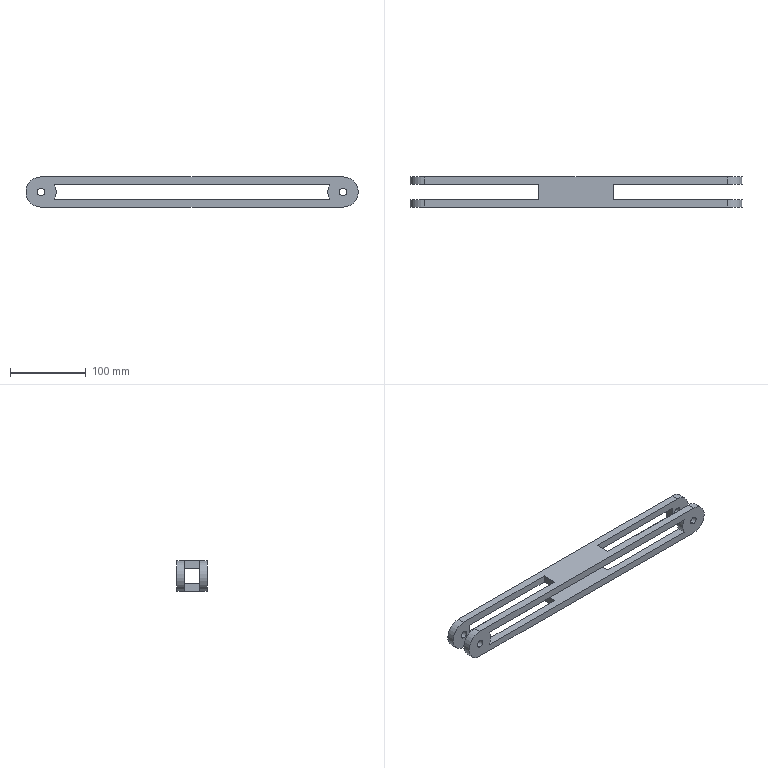Part | SolidWorks | features ICE 4, MirrorPattern 2, Extrusion 1 | 1 solid | 30 faces | box 440 x 40 x 40 mm | volume 233504 mm3 | plane 16 | cylinder 14 | commonest cylinder face diameters 10 x8 40 x6
STEP:
#1=CARTESIAN_POINT('',(-200.,-20.,-5.));
#2=VERTEX_POINT('',#1);
#3=CARTESIAN_POINT('',(-200.,-20.,5.));
#4=VERTEX_POINT('',#3);
#5=CARTESIAN_POINT('',(-200.,-20.,0.));
#6=DIRECTION('',(0.,1.,0.));
#7=DIRECTION('',(0.,0.,-1.));
#8=AXIS2_PLACEMENT_3D('',#5,#6,#7);
#9=CIRCLE('',#8,5.);
#10=EDGE_CURVE('',#2,#4,#9,.T.);
#11=ORIENTED_EDGE('',*,*,#10,.F.);
#12=CARTESIAN_POINT('',(-200.,-10.,-5.));
#13=VERTEX_POINT('',#12);
#14=CARTESIAN_POINT('',(-200.,0.,-5.));
#15=DIRECTION('',(0.,1.,0.));
#16=VECTOR('',#15,1000.);
#17=LINE('',#14,#16);
#18=EDGE_CURVE('',#2,#13,#17,.T.);
#19=ORIENTED_EDGE('',*,*,#18,.T.);
#20=CARTESIAN_POINT('',(-200.,-10.,5.));
#21=VERTEX_POINT('',#20);
#22=CARTESIAN_POINT('',(-200.,-10.,0.));
#23=DIRECTION('',(0.,-1.,0.));
#24=DIRECTION('',(0.,0.,1.));
#25=AXIS2_PLACEMENT_3D('',#22,#23,#24);
#26=CIRCLE('',#25,5.);
#27=EDGE_CURVE('',#21,#13,#26,.T.);
#28=ORIENTED_EDGE('',*,*,#27,.F.);
#29=CARTESIAN_POINT('',(-200.,0.,5.));
#30=DIRECTION('',(0.,1.,0.));
#31=VECTOR('',#30,1000.);
#32=LINE('',#29,#31);
#33=EDGE_CURVE('',#4,#21,#32,.T.);
#34=ORIENTED_EDGE('',*,*,#33,.F.);
#35=EDGE_LOOP('',(#11,#19,#28,#34));
#36=FACE_OUTER_BOUND('',#35,.T.);
#37=CARTESIAN_POINT('',(-200.,0.,0.));
#38=DIRECTION('',(0.,1.,0.));
#39=DIRECTION('',(0.,0.,1.));
#40=AXIS2_PLACEMENT_3D('',#37,#38,#39);
#41=CYLINDRICAL_SURFACE('',#40,5.);
#42=ADVANCED_FACE('',(#36),#41,.F.);
#43=CARTESIAN_POINT('',(-200.,10.,5.));
#44=VERTEX_POINT('',#43);
#45=CARTESIAN_POINT('',(-200.,10.,-5.));
#46=VERTEX_POINT('',#45);
#47=CARTESIAN_POINT('',(-200.,10.,0.));
#48=DIRECTION('',(0.,-1.,0.));
#49=DIRECTION('',(0.,0.,-1.));
#50=AXIS2_PLACEMENT_3D('',#47,#48,#49);
#51=CIRCLE('',#50,5.);
#52=EDGE_CURVE('',#44,#46,#51,.T.);
#53=ORIENTED_EDGE('',*,*,#52,.T.);
#54=CARTESIAN_POINT('',(-200.,20.,-5.));
#55=VERTEX_POINT('',#54);
#56=CARTESIAN_POINT('',(-200.,0.,-5.));
#57=DIRECTION('',(0.,1.,0.));
#58=VECTOR('',#57,1000.);
#59=LINE('',#56,#58);
#60=EDGE_CURVE('',#46,#55,#59,.T.);
#61=ORIENTED_EDGE('',*,*,#60,.T.);
#62=CARTESIAN_POINT('',(-200.,20.,5.));
#63=VERTEX_POINT('',#62);
#64=CARTESIAN_POINT('',(-200.,20.,0.));
#65=DIRECTION('',(0.,1.,0.));
#66=DIRECTION('',(0.,0.,-1.));
#67=AXIS2_PLACEMENT_3D('',#64,#65,#66);
#68=CIRCLE('',#67,5.);
#69=EDGE_CURVE('',#55,#63,#68,.T.);
#70=ORIENTED_EDGE('',*,*,#69,.T.);
#71=CARTESIAN_POINT('',(-200.,0.,5.));
#72=DIRECTION('',(0.,1.,0.));
#73=VECTOR('',#72,1000.);
#74=LINE('',#71,#73);
#75=EDGE_CURVE('',#44,#63,#74,.T.);
#76=ORIENTED_EDGE('',*,*,#75,.F.);
#77=EDGE_LOOP('',(#53,#61,#70,#76));
#78=FACE_OUTER_BOUND('',#77,.T.);
#79=CARTESIAN_POINT('',(-200.,0.,0.));
#80=DIRECTION('',(0.,1.,0.));
#81=DIRECTION('',(0.,0.,1.));
#82=AXIS2_PLACEMENT_3D('',#79,#80,#81);
#83=CYLINDRICAL_SURFACE('',#82,5.);
#84=ADVANCED_FACE('',(#78),#83,.F.);
#85=CARTESIAN_POINT('',(200.,10.,-5.));
#86=VERTEX_POINT('',#85);
#87=CARTESIAN_POINT('',(200.,10.,5.));
#88=VERTEX_POINT('',#87);
#89=CARTESIAN_POINT('',(200.,10.,0.));
#90=DIRECTION('',(0.,1.,0.));
#91=DIRECTION('',(0.,0.,1.));
#92=AXIS2_PLACEMENT_3D('',#89,#90,#91);
#93=CIRCLE('',#92,5.);
#94=EDGE_CURVE('',#86,#88,#93,.T.);
#95=ORIENTED_EDGE('',*,*,#94,.F.);
#96=CARTESIAN_POINT('',(200.,20.,-5.));
#97=VERTEX_POINT('',#96);
#98=CARTESIAN_POINT('',(200.,0.,-5.));
#99=DIRECTION('',(0.,1.,0.));
#100=VECTOR('',#99,1000.);
#101=LINE('',#98,#100);
#102=EDGE_CURVE('',#86,#97,#101,.T.);
#103=ORIENTED_EDGE('',*,*,#102,.T.);
#104=CARTESIAN_POINT('',(200.,20.,5.));
#105=VERTEX_POINT('',#104);
#106=CARTESIAN_POINT('',(200.,20.,0.));
#107=DIRECTION('',(0.,1.,0.));
#108=DIRECTION('',(0.,0.,1.));
#109=AXIS2_PLACEMENT_3D('',#106,#107,#108);
#110=CIRCLE('',#109,5.);
#111=EDGE_CURVE('',#97,#105,#110,.T.);
#112=ORIENTED_EDGE('',*,*,#111,.T.);
#113=CARTESIAN_POINT('',(200.,0.,5.));
#114=DIRECTION('',(0.,1.,0.));
#115=VECTOR('',#114,1000.);
#116=LINE('',#113,#115);
#117=EDGE_CURVE('',#88,#105,#116,.T.);
#118=ORIENTED_EDGE('',*,*,#117,.F.);
#119=EDGE_LOOP('',(#95,#103,#112,#118));
#120=FACE_OUTER_BOUND('',#119,.T.);
#121=CARTESIAN_POINT('',(200.,0.,0.));
#122=DIRECTION('',(0.,1.,0.));
#123=DIRECTION('',(0.,0.,1.));
#124=AXIS2_PLACEMENT_3D('',#121,#122,#123);
#125=CYLINDRICAL_SURFACE('',#124,5.);
#126=ADVANCED_FACE('',(#120),#125,.F.);
#127=CARTESIAN_POINT('',(200.,-20.,-5.));
#128=VERTEX_POINT('',#127);
#129=CARTESIAN_POINT('',(200.,-20.,5.));
#130=VERTEX_POINT('',#129);
#131=CARTESIAN_POINT('',(200.,-20.,0.));
#132=DIRECTION('',(0.,1.,0.));
#133=DIRECTION('',(0.,0.,1.));
#134=AXIS2_PLACEMENT_3D('',#131,#132,#133);
#135=CIRCLE('',#134,5.);
#136=EDGE_CURVE('',#128,#130,#135,.T.);
#137=ORIENTED_EDGE('',*,*,#136,.F.);
#138=CARTESIAN_POINT('',(200.,-10.,-5.));
#139=VERTEX_POINT('',#138);
#140=CARTESIAN_POINT('',(200.,0.,-5.));
#141=DIRECTION('',(0.,1.,0.));
#142=VECTOR('',#141,1000.);
#143=LINE('',#140,#142);
#144=EDGE_CURVE('',#128,#139,#143,.T.);
#145=ORIENTED_EDGE('',*,*,#144,.T.);
#146=CARTESIAN_POINT('',(200.,-10.,5.));
#147=VERTEX_POINT('',#146);
#148=CARTESIAN_POINT('',(200.,-10.,0.));
#149=DIRECTION('',(0.,1.,0.));
#150=DIRECTION('',(0.,0.,-1.));
#151=AXIS2_PLACEMENT_3D('',#148,#149,#150);
#152=CIRCLE('',#151,5.);
#153=EDGE_CURVE('',#139,#147,#152,.T.);
#154=ORIENTED_EDGE('',*,*,#153,.T.);
#155=CARTESIAN_POINT('',(200.,0.,5.));
#156=DIRECTION('',(0.,1.,0.));
#157=VECTOR('',#156,1000.);
#158=LINE('',#155,#157);
#159=EDGE_CURVE('',#130,#147,#158,.T.);
#160=ORIENTED_EDGE('',*,*,#159,.F.);
#161=EDGE_LOOP('',(#137,#145,#154,#160));
#162=FACE_OUTER_BOUND('',#161,.T.);
#163=CARTESIAN_POINT('',(200.,0.,0.));
#164=DIRECTION('',(0.,1.,0.));
#165=DIRECTION('',(0.,0.,1.));
#166=AXIS2_PLACEMENT_3D('',#163,#164,#165);
#167=CYLINDRICAL_SURFACE('',#166,5.);
#168=ADVANCED_FACE('',(#162),#167,.F.);
#169=CARTESIAN_POINT('',(182.679,-10.,10.));
#170=VERTEX_POINT('',#169);
#171=CARTESIAN_POINT('',(49.825,-10.,10.));
#172=VERTEX_POINT('',#171);
#173=CARTESIAN_POINT('',(-190.,-10.,10.));
#174=DIRECTION('',(-1.,0.,0.));
#175=VECTOR('',#174,1000.);
#176=LINE('',#173,#175);
#177=EDGE_CURVE('',#170,#172,#176,.T.);
#178=ORIENTED_EDGE('',*,*,#177,.F.);
#179=CARTESIAN_POINT('',(182.679,-20.,10.));
#180=VERTEX_POINT('',#179);
#181=CARTESIAN_POINT('',(182.679,-10.,10.));
#182=DIRECTION('',(0.,1.,0.));
#183=VECTOR('',#182,1000.);
#184=LINE('',#181,#183);
#185=EDGE_CURVE('',#180,#170,#184,.T.);
#186=ORIENTED_EDGE('',*,*,#185,.F.);
#187=CARTESIAN_POINT('',(-182.679,-20.,10.));
#188=VERTEX_POINT('',#187);
#189=CARTESIAN_POINT('',(-190.,-20.,10.));
#190=DIRECTION('',(1.,0.,0.));
#191=VECTOR('',#190,1000.);
#192=LINE('',#189,#191);
#193=EDGE_CURVE('',#188,#180,#192,.T.);
#194=ORIENTED_EDGE('',*,*,#193,.F.);
#195=CARTESIAN_POINT('',(-182.679,-10.,10.));
#196=VERTEX_POINT('',#195);
#197=CARTESIAN_POINT('',(-182.679,-10.,10.));
#198=DIRECTION('',(0.,-1.,0.));
#199=VECTOR('',#198,1000.);
#200=LINE('',#197,#199);
#201=EDGE_CURVE('',#196,#188,#200,.T.);
#202=ORIENTED_EDGE('',*,*,#201,.F.);
#203=CARTESIAN_POINT('',(-49.825,-10.,10.));
#204=VERTEX_POINT('',#203);
#205=CARTESIAN_POINT('',(-190.,-10.,10.));
#206=DIRECTION('',(1.,0.,0.));
#207=VECTOR('',#206,1000.);
#208=LINE('',#205,#207);
#209=EDGE_CURVE('',#196,#204,#208,.T.);
#210=ORIENTED_EDGE('',*,*,#209,.T.);
#211=CARTESIAN_POINT('',(-49.825,10.,10.));
#212=VERTEX_POINT('',#211);
#213=CARTESIAN_POINT('',(-49.825,0.,10.));
#214=DIRECTION('',(0.,1.,0.));
#215=VECTOR('',#214,1000.);
#216=LINE('',#213,#215);
#217=EDGE_CURVE('',#204,#212,#216,.T.);
#218=ORIENTED_EDGE('',*,*,#217,.T.);
#219=CARTESIAN_POINT('',(-190.,10.,10.));
#220=VERTEX_POINT('',#219);
#221=CARTESIAN_POINT('',(-190.,10.,10.));
#222=DIRECTION('',(-1.,0.,0.));
#223=VECTOR('',#222,1000.);
#224=LINE('',#221,#223);
#225=EDGE_CURVE('',#212,#220,#224,.T.);
#226=ORIENTED_EDGE('',*,*,#225,.T.);
#227=CARTESIAN_POINT('',(-190.,20.,10.));
#228=VERTEX_POINT('',#227);
#229=CARTESIAN_POINT('',(-190.,0.,10.));
#230=DIRECTION('',(0.,1.,0.));
#231=VECTOR('',#230,1000.);
#232=LINE('',#229,#231);
#233=EDGE_CURVE('',#220,#228,#232,.T.);
#234=ORIENTED_EDGE('',*,*,#233,.T.);
#235=CARTESIAN_POINT('',(190.,20.,10.));
#236=VERTEX_POINT('',#235);
#237=CARTESIAN_POINT('',(-190.,20.,10.));
#238=DIRECTION('',(1.,0.,0.));
#239=VECTOR('',#238,1000.);
#240=LINE('',#237,#239);
#241=EDGE_CURVE('',#228,#236,#240,.T.);
#242=ORIENTED_EDGE('',*,*,#241,.T.);
#243=CARTESIAN_POINT('',(190.,10.,10.));
#244=VERTEX_POINT('',#243);
#245=CARTESIAN_POINT('',(190.,0.,10.));
#246=DIRECTION('',(0.,1.,0.));
#247=VECTOR('',#246,1000.);
#248=LINE('',#245,#247);
#249=EDGE_CURVE('',#244,#236,#248,.T.);
#250=ORIENTED_EDGE('',*,*,#249,.F.);
#251=CARTESIAN_POINT('',(49.825,10.,10.));
#252=VERTEX_POINT('',#251);
#253=CARTESIAN_POINT('',(-190.,10.,10.));
#254=DIRECTION('',(1.,0.,0.));
#255=VECTOR('',#254,1000.);
#256=LINE('',#253,#255);
#257=EDGE_CURVE('',#252,#244,#256,.T.);
#258=ORIENTED_EDGE('',*,*,#257,.F.);
#259=CARTESIAN_POINT('',(49.825,0.,10.));
#260=DIRECTION('',(0.,1.,0.));
#261=VECTOR('',#260,1000.);
#262=LINE('',#259,#261);
#263=EDGE_CURVE('',#172,#252,#262,.T.);
#264=ORIENTED_EDGE('',*,*,#263,.F.);
#265=EDGE_LOOP('',(#178,#186,#194,#202,#210,#218,#226,#234,#242,#250,#258,#264));
#266=FACE_OUTER_BOUND('',#265,.T.);
#267=CARTESIAN_POINT('',(-190.,0.,10.));
#268=DIRECTION('',(0.,0.,1.));
#269=DIRECTION('',(1.,0.,0.));
#270=AXIS2_PLACEMENT_3D('',#267,#268,#269);
#271=PLANE('',#270);
#272=ADVANCED_FACE('',(#266),#271,.F.);
#273=CARTESIAN_POINT('',(49.825,-10.,-10.));
#274=VERTEX_POINT('',#273);
#275=CARTESIAN_POINT('',(182.679,-10.,-10.));
#276=VERTEX_POINT('',#275);
#277=CARTESIAN_POINT('',(190.,-10.,-10.));
#278=DIRECTION('',(1.,0.,0.));
#279=VECTOR('',#278,1000.);
#280=LINE('',#277,#279);
#281=EDGE_CURVE('',#274,#276,#280,.T.);
#282=ORIENTED_EDGE('',*,*,#281,.F.);
#283=CARTESIAN_POINT('',(49.825,10.,-10.));
#284=VERTEX_POINT('',#283);
#285=CARTESIAN_POINT('',(49.825,0.,-10.));
#286=DIRECTION('',(0.,-1.,0.));
#287=VECTOR('',#286,1000.);
#288=LINE('',#285,#287);
#289=EDGE_CURVE('',#284,#274,#288,.T.);
#290=ORIENTED_EDGE('',*,*,#289,.F.);
#291=CARTESIAN_POINT('',(190.,10.,-10.));
#292=VERTEX_POINT('',#291);
#293=CARTESIAN_POINT('',(190.,10.,-10.));
#294=DIRECTION('',(-1.,0.,0.));
#295=VECTOR('',#294,1000.);
#296=LINE('',#293,#295);
#297=EDGE_CURVE('',#292,#284,#296,.T.);
#298=ORIENTED_EDGE('',*,*,#297,.F.);
#299=CARTESIAN_POINT('',(190.,20.,-10.));
#300=VERTEX_POINT('',#299);
#301=CARTESIAN_POINT('',(190.,0.,-10.));
#302=DIRECTION('',(0.,1.,0.));
#303=VECTOR('',#302,1000.);
#304=LINE('',#301,#303);
#305=EDGE_CURVE('',#292,#300,#304,.T.);
#306=ORIENTED_EDGE('',*,*,#305,.T.);
#307=CARTESIAN_POINT('',(-190.,20.,-10.));
#308=VERTEX_POINT('',#307);
#309=CARTESIAN_POINT('',(190.,20.,-10.));
#310=DIRECTION('',(-1.,0.,0.));
#311=VECTOR('',#310,1000.);
#312=LINE('',#309,#311);
#313=EDGE_CURVE('',#300,#308,#312,.T.);
#314=ORIENTED_EDGE('',*,*,#313,.T.);
#315=CARTESIAN_POINT('',(-190.,10.,-10.));
#316=VERTEX_POINT('',#315);
#317=CARTESIAN_POINT('',(-190.,0.,-10.));
#318=DIRECTION('',(0.,1.,0.));
#319=VECTOR('',#318,1000.);
#320=LINE('',#317,#319);
#321=EDGE_CURVE('',#316,#308,#320,.T.);
#322=ORIENTED_EDGE('',*,*,#321,.F.);
#323=CARTESIAN_POINT('',(-49.825,10.,-10.));
#324=VERTEX_POINT('',#323);
#325=CARTESIAN_POINT('',(190.,10.,-10.));
#326=DIRECTION('',(1.,0.,0.));
#327=VECTOR('',#326,1000.);
#328=LINE('',#325,#327);
#329=EDGE_CURVE('',#316,#324,#328,.T.);
#330=ORIENTED_EDGE('',*,*,#329,.T.);
#331=CARTESIAN_POINT('',(-49.825,-10.,-10.));
#332=VERTEX_POINT('',#331);
#333=CARTESIAN_POINT('',(-49.825,0.,-10.));
#334=DIRECTION('',(0.,-1.,0.));
#335=VECTOR('',#334,1000.);
#336=LINE('',#333,#335);
#337=EDGE_CURVE('',#324,#332,#336,.T.);
#338=ORIENTED_EDGE('',*,*,#337,.T.);
#339=CARTESIAN_POINT('',(-182.679,-10.,-10.));
#340=VERTEX_POINT('',#339);
#341=CARTESIAN_POINT('',(190.,-10.,-10.));
#342=DIRECTION('',(-1.,0.,0.));
#343=VECTOR('',#342,1000.);
#344=LINE('',#341,#343);
#345=EDGE_CURVE('',#332,#340,#344,.T.);
#346=ORIENTED_EDGE('',*,*,#345,.T.);
#347=CARTESIAN_POINT('',(-182.679,-20.,-10.));
#348=VERTEX_POINT('',#347);
#349=CARTESIAN_POINT('',(-182.679,-10.,-10.));
#350=DIRECTION('',(0.,1.,0.));
#351=VECTOR('',#350,1000.);
#352=LINE('',#349,#351);
#353=EDGE_CURVE('',#348,#340,#352,.T.);
#354=ORIENTED_EDGE('',*,*,#353,.F.);
#355=CARTESIAN_POINT('',(182.679,-20.,-10.));
#356=VERTEX_POINT('',#355);
#357=CARTESIAN_POINT('',(190.,-20.,-10.));
#358=DIRECTION('',(-1.,0.,0.));
#359=VECTOR('',#358,1000.);
#360=LINE('',#357,#359);
#361=EDGE_CURVE('',#356,#348,#360,.T.);
#362=ORIENTED_EDGE('',*,*,#361,.F.);
#363=CARTESIAN_POINT('',(182.679,-10.,-10.));
#364=DIRECTION('',(0.,-1.,0.));
#365=VECTOR('',#364,1000.);
#366=LINE('',#363,#365);
#367=EDGE_CURVE('',#276,#356,#366,.T.);
#368=ORIENTED_EDGE('',*,*,#367,.F.);
#369=EDGE_LOOP('',(#282,#290,#298,#306,#314,#322,#330,#338,#346,#354,#362,#368));
#370=FACE_OUTER_BOUND('',#369,.T.);
#371=CARTESIAN_POINT('',(190.,0.,-10.));
#372=DIRECTION('',(0.,0.,-1.));
#373=DIRECTION('',(-1.,0.,0.));
#374=AXIS2_PLACEMENT_3D('',#371,#372,#373);
#375=PLANE('',#374);
#376=ADVANCED_FACE('',(#370),#375,.F.);
#377=CARTESIAN_POINT('',(190.,10.,10.));
#378=DIRECTION('',(0.,0.,-1.));
#379=VECTOR('',#378,1000.);
#380=LINE('',#377,#379);
#381=EDGE_CURVE('',#244,#292,#380,.T.);
#382=ORIENTED_EDGE('',*,*,#381,.F.);
#383=ORIENTED_EDGE('',*,*,#249,.T.);
#384=CARTESIAN_POINT('',(190.,20.,10.));
#385=DIRECTION('',(0.,0.,-1.));
#386=VECTOR('',#385,1000.);
#387=LINE('',#384,#386);
#388=EDGE_CURVE('',#236,#300,#387,.T.);
#389=ORIENTED_EDGE('',*,*,#388,.T.);
#390=ORIENTED_EDGE('',*,*,#305,.F.);
#391=EDGE_LOOP('',(#382,#383,#389,#390));
#392=FACE_OUTER_BOUND('',#391,.T.);
#393=CARTESIAN_POINT('',(190.,0.,10.));
#394=DIRECTION('',(1.,0.,0.));
#395=DIRECTION('',(0.,0.,-1.));
#396=AXIS2_PLACEMENT_3D('',#393,#394,#395);
#397=PLANE('',#396);
#398=ADVANCED_FACE('',(#392),#397,.F.);
#399=CARTESIAN_POINT('',(200.,-10.,-20.));
#400=VERTEX_POINT('',#399);
#401=CARTESIAN_POINT('',(49.825,-10.,-20.));
#402=VERTEX_POINT('',#401);
#403=CARTESIAN_POINT('',(200.,-10.,-20.));
#404=DIRECTION('',(-1.,0.,0.));
#405=VECTOR('',#404,1000.);
#406=LINE('',#403,#405);
#407=EDGE_CURVE('',#400,#402,#406,.T.);
#408=ORIENTED_EDGE('',*,*,#407,.F.);
#409=CARTESIAN_POINT('',(200.,-20.,-20.));
#410=VERTEX_POINT('',#409);
#411=CARTESIAN_POINT('',(200.,-10.,-20.));
#412=DIRECTION('',(0.,1.,0.));
#413=VECTOR('',#412,1000.);
#414=LINE('',#411,#413);
#415=EDGE_CURVE('',#410,#400,#414,.T.);
#416=ORIENTED_EDGE('',*,*,#415,.F.);
#417=CARTESIAN_POINT('',(-200.,-20.,-20.));
#418=VERTEX_POINT('',#417);
#419=CARTESIAN_POINT('',(-200.,-20.,-20.));
#420=DIRECTION('',(-1.,0.,0.));
#421=VECTOR('',#420,1000.);
#422=LINE('',#419,#421);
#423=EDGE_CURVE('',#410,#418,#422,.T.);
#424=ORIENTED_EDGE('',*,*,#423,.T.);
#425=CARTESIAN_POINT('',(-200.,-10.,-20.));
#426=VERTEX_POINT('',#425);
#427=CARTESIAN_POINT('',(-200.,-10.,-20.));
#428=DIRECTION('',(0.,-1.,0.));
#429=VECTOR('',#428,1000.);
#430=LINE('',#427,#429);
#431=EDGE_CURVE('',#426,#418,#430,.T.);
#432=ORIENTED_EDGE('',*,*,#431,.F.);
#433=CARTESIAN_POINT('',(-49.825,-10.,-20.));
#434=VERTEX_POINT('',#433);
#435=CARTESIAN_POINT('',(-200.,-10.,-20.));
#436=DIRECTION('',(1.,0.,0.));
#437=VECTOR('',#436,1000.);
#438=LINE('',#435,#437);
#439=EDGE_CURVE('',#426,#434,#438,.T.);
#440=ORIENTED_EDGE('',*,*,#439,.T.);
#441=CARTESIAN_POINT('',(-49.825,10.,-20.));
#442=VERTEX_POINT('',#441);
#443=CARTESIAN_POINT('',(-49.825,10.,-20.));
#444=DIRECTION('',(0.,1.,0.));
#445=VECTOR('',#444,1000.);
#446=LINE('',#443,#445);
#447=EDGE_CURVE('',#434,#442,#446,.T.);
#448=ORIENTED_EDGE('',*,*,#447,.T.);
#449=CARTESIAN_POINT('',(-200.,10.,-20.));
#450=VERTEX_POINT('',#449);
#451=CARTESIAN_POINT('',(-200.,10.,-20.));
#452=DIRECTION('',(-1.,0.,0.));
#453=VECTOR('',#452,1000.);
#454=LINE('',#451,#453);
#455=EDGE_CURVE('',#442,#450,#454,.T.);
#456=ORIENTED_EDGE('',*,*,#455,.T.);
#457=CARTESIAN_POINT('',(-200.,20.,-20.));
#458=VERTEX_POINT('',#457);
#459=CARTESIAN_POINT('',(-200.,20.,-20.));
#460=DIRECTION('',(0.,-1.,0.));
#461=VECTOR('',#460,1000.);
#462=LINE('',#459,#461);
#463=EDGE_CURVE('',#458,#450,#462,.T.);
#464=ORIENTED_EDGE('',*,*,#463,.F.);
#465=CARTESIAN_POINT('',(200.,20.,-20.));
#466=VERTEX_POINT('',#465);
#467=CARTESIAN_POINT('',(-200.,20.,-20.));
#468=DIRECTION('',(-1.,0.,0.));
#469=VECTOR('',#468,1000.);
#470=LINE('',#467,#469);
#471=EDGE_CURVE('',#466,#458,#470,.T.);
#472=ORIENTED_EDGE('',*,*,#471,.F.);
#473=CARTESIAN_POINT('',(200.,10.,-20.));
#474=VERTEX_POINT('',#473);
#475=CARTESIAN_POINT('',(200.,20.,-20.));
#476=DIRECTION('',(0.,-1.,0.));
#477=VECTOR('',#476,1000.);
#478=LINE('',#475,#477);
#479=EDGE_CURVE('',#466,#474,#478,.T.);
#480=ORIENTED_EDGE('',*,*,#479,.T.);
#481=CARTESIAN_POINT('',(49.825,10.,-20.));
#482=VERTEX_POINT('',#481);
#483=CARTESIAN_POINT('',(200.,10.,-20.));
#484=DIRECTION('',(1.,0.,0.));
#485=VECTOR('',#484,1000.);
#486=LINE('',#483,#485);
#487=EDGE_CURVE('',#482,#474,#486,.T.);
#488=ORIENTED_EDGE('',*,*,#487,.F.);
#489=CARTESIAN_POINT('',(49.825,10.,-20.));
#490=DIRECTION('',(0.,1.,0.));
#491=VECTOR('',#490,1000.);
#492=LINE('',#489,#491);
#493=EDGE_CURVE('',#402,#482,#492,.T.);
#494=ORIENTED_EDGE('',*,*,#493,.F.);
#495=EDGE_LOOP('',(#408,#416,#424,#432,#440,#448,#456,#464,#472,#480,#488,#494));
#496=FACE_OUTER_BOUND('',#495,.T.);
#497=CARTESIAN_POINT('',(-200.,20.,-20.));
#498=DIRECTION('',(0.,0.,1.));
#499=DIRECTION('',(1.,0.,0.));
#500=AXIS2_PLACEMENT_3D('',#497,#498,#499);
#501=PLANE('',#500);
#502=ADVANCED_FACE('',(#496),#501,.F.);
#503=CARTESIAN_POINT('',(200.,-10.,20.));
#504=VERTEX_POINT('',#503);
#505=CARTESIAN_POINT('',(49.825,-10.,20.));
#506=VERTEX_POINT('',#505);
#507=CARTESIAN_POINT('',(200.,-10.,20.));
#508=DIRECTION('',(-1.,0.,0.));
#509=VECTOR('',#508,1000.);
#510=LINE('',#507,#509);
#511=EDGE_CURVE('',#504,#506,#510,.T.);
#512=ORIENTED_EDGE('',*,*,#511,.T.);
#513=CARTESIAN_POINT('',(49.825,10.,20.));
#514=VERTEX_POINT('',#513);
#515=CARTESIAN_POINT('',(49.825,10.,20.));
#516=DIRECTION('',(0.,1.,0.));
#517=VECTOR('',#516,1000.);
#518=LINE('',#515,#517);
#519=EDGE_CURVE('',#506,#514,#518,.T.);
#520=ORIENTED_EDGE('',*,*,#519,.T.);
#521=CARTESIAN_POINT('',(200.,10.,20.));
#522=VERTEX_POINT('',#521);
#523=CARTESIAN_POINT('',(200.,10.,20.));
#524=DIRECTION('',(1.,0.,0.));
#525=VECTOR('',#524,1000.);
#526=LINE('',#523,#525);
#527=EDGE_CURVE('',#514,#522,#526,.T.);
#528=ORIENTED_EDGE('',*,*,#527,.T.);
#529=CARTESIAN_POINT('',(200.,20.,20.));
#530=VERTEX_POINT('',#529);
#531=CARTESIAN_POINT('',(200.,20.,20.));
#532=DIRECTION('',(0.,-1.,0.));
#533=VECTOR('',#532,1000.);
#534=LINE('',#531,#533);
#535=EDGE_CURVE('',#530,#522,#534,.T.);
#536=ORIENTED_EDGE('',*,*,#535,.F.);
#537=CARTESIAN_POINT('',(-200.,20.,20.));
#538=VERTEX_POINT('',#537);
#539=CARTESIAN_POINT('',(-200.,20.,20.));
#540=DIRECTION('',(1.,0.,0.));
#541=VECTOR('',#540,1000.);
#542=LINE('',#539,#541);
#543=EDGE_CURVE('',#538,#530,#542,.T.);
#544=ORIENTED_EDGE('',*,*,#543,.F.);
#545=CARTESIAN_POINT('',(-200.,10.,20.));
#546=VERTEX_POINT('',#545);
#547=CARTESIAN_POINT('',(-200.,20.,20.));
#548=DIRECTION('',(0.,-1.,0.));
#549=VECTOR('',#548,1000.);
#550=LINE('',#547,#549);
#551=EDGE_CURVE('',#538,#546,#550,.T.);
#552=ORIENTED_EDGE('',*,*,#551,.T.);
#553=CARTESIAN_POINT('',(-49.825,10.,20.));
#554=VERTEX_POINT('',#553);
#555=CARTESIAN_POINT('',(-200.,10.,20.));
#556=DIRECTION('',(-1.,0.,0.));
#557=VECTOR('',#556,1000.);
#558=LINE('',#555,#557);
#559=EDGE_CURVE('',#554,#546,#558,.T.);
#560=ORIENTED_EDGE('',*,*,#559,.F.);
#561=CARTESIAN_POINT('',(-49.825,-10.,20.));
#562=VERTEX_POINT('',#561);
#563=CARTESIAN_POINT('',(-49.825,10.,20.));
#564=DIRECTION('',(0.,1.,0.));
#565=VECTOR('',#564,1000.);
#566=LINE('',#563,#565);
#567=EDGE_CURVE('',#562,#554,#566,.T.);
#568=ORIENTED_EDGE('',*,*,#567,.F.);
#569=CARTESIAN_POINT('',(-200.,-10.,20.));
#570=VERTEX_POINT('',#569);
#571=CARTESIAN_POINT('',(-200.,-10.,20.));
#572=DIRECTION('',(1.,0.,0.));
#573=VECTOR('',#572,1000.);
#574=LINE('',#571,#573);
#575=EDGE_CURVE('',#570,#562,#574,.T.);
#576=ORIENTED_EDGE('',*,*,#575,.F.);
#577=CARTESIAN_POINT('',(-200.,-20.,20.));
#578=VERTEX_POINT('',#577);
#579=CARTESIAN_POINT('',(-200.,20.,20.));
#580=DIRECTION('',(0.,-1.,0.));
#581=VECTOR('',#580,1000.);
#582=LINE('',#579,#581);
#583=EDGE_CURVE('',#570,#578,#582,.T.);
#584=ORIENTED_EDGE('',*,*,#583,.T.);
#585=CARTESIAN_POINT('',(200.,-20.,20.));
#586=VERTEX_POINT('',#585);
#587=CARTESIAN_POINT('',(-200.,-20.,20.));
#588=DIRECTION('',(1.,0.,0.));
#589=VECTOR('',#588,1000.);
#590=LINE('',#587,#589);
#591=EDGE_CURVE('',#578,#586,#590,.T.);
#592=ORIENTED_EDGE('',*,*,#591,.T.);
#593=CARTESIAN_POINT('',(200.,-10.,20.));
#594=DIRECTION('',(0.,1.,0.));
#595=VECTOR('',#594,1000.);
#596=LINE('',#593,#595);
#597=EDGE_CURVE('',#586,#504,#596,.T.);
#598=ORIENTED_EDGE('',*,*,#597,.T.);
#599=EDGE_LOOP('',(#512,#520,#528,#536,#544,#552,#560,#568,#576,#584,#592,#598));
#600=FACE_OUTER_BOUND('',#599,.T.);
#601=CARTESIAN_POINT('',(-200.,20.,20.));
#602=DIRECTION('',(0.,0.,-1.));
#603=DIRECTION('',(-1.,0.,0.));
#604=AXIS2_PLACEMENT_3D('',#601,#602,#603);
#605=PLANE('',#604);
#606=ADVANCED_FACE('',(#600),#605,.F.);
#607=ORIENTED_EDGE('',*,*,#144,.F.);
#608=CARTESIAN_POINT('',(200.,-20.,0.));
#609=DIRECTION('',(0.,1.,0.));
#610=DIRECTION('',(0.,0.,1.));
#611=AXIS2_PLACEMENT_3D('',#608,#609,#610);
#612=CIRCLE('',#611,5.);
#613=EDGE_CURVE('',#130,#128,#612,.T.);
#614=ORIENTED_EDGE('',*,*,#613,.F.);
#615=ORIENTED_EDGE('',*,*,#159,.T.);
#616=CARTESIAN_POINT('',(200.,-10.,0.));
#617=DIRECTION('',(0.,1.,0.));
#618=DIRECTION('',(0.,0.,-1.));
#619=AXIS2_PLACEMENT_3D('',#616,#617,#618);
#620=CIRCLE('',#619,5.);
#621=EDGE_CURVE('',#147,#139,#620,.T.);
#622=ORIENTED_EDGE('',*,*,#621,.T.);
#623=EDGE_LOOP('',(#607,#614,#615,#622));
#624=FACE_OUTER_BOUND('',#623,.T.);
#625=CARTESIAN_POINT('',(200.,0.,0.));
#626=DIRECTION('',(0.,1.,0.));
#627=DIRECTION('',(0.,0.,1.));
#628=AXIS2_PLACEMENT_3D('',#625,#626,#627);
#629=CYLINDRICAL_SURFACE('',#628,5.);
#630=ADVANCED_FACE('',(#624),#629,.F.);
#631=ORIENTED_EDGE('',*,*,#102,.F.);
#632=CARTESIAN_POINT('',(200.,10.,0.));
#633=DIRECTION('',(0.,1.,0.));
#634=DIRECTION('',(0.,0.,1.));
#635=AXIS2_PLACEMENT_3D('',#632,#633,#634);
#636=CIRCLE('',#635,5.);
#637=EDGE_CURVE('',#88,#86,#636,.T.);
#638=ORIENTED_EDGE('',*,*,#637,.F.);
#639=ORIENTED_EDGE('',*,*,#117,.T.);
#640=CARTESIAN_POINT('',(200.,20.,0.));
#641=DIRECTION('',(0.,1.,0.));
#642=DIRECTION('',(0.,0.,1.));
#643=AXIS2_PLACEMENT_3D('',#640,#641,#642);
#644=CIRCLE('',#643,5.);
#645=EDGE_CURVE('',#105,#97,#644,.T.);
#646=ORIENTED_EDGE('',*,*,#645,.T.);
#647=EDGE_LOOP('',(#631,#638,#639,#646));
#648=FACE_OUTER_BOUND('',#647,.T.);
#649=CARTESIAN_POINT('',(200.,0.,0.));
#650=DIRECTION('',(0.,1.,0.));
#651=DIRECTION('',(0.,0.,1.));
#652=AXIS2_PLACEMENT_3D('',#649,#650,#651);
#653=CYLINDRICAL_SURFACE('',#652,5.);
#654=ADVANCED_FACE('',(#648),#653,.F.);
#655=ORIENTED_EDGE('',*,*,#60,.F.);
#656=CARTESIAN_POINT('',(-200.,10.,0.));
#657=DIRECTION('',(0.,-1.,0.));
#658=DIRECTION('',(0.,0.,-1.));
#659=AXIS2_PLACEMENT_3D('',#656,#657,#658);
#660=CIRCLE('',#659,5.);
#661=EDGE_CURVE('',#46,#44,#660,.T.);
#662=ORIENTED_EDGE('',*,*,#661,.T.);
#663=ORIENTED_EDGE('',*,*,#75,.T.);
#664=CARTESIAN_POINT('',(-200.,20.,0.));
#665=DIRECTION('',(0.,1.,0.));
#666=DIRECTION('',(0.,0.,-1.));
#667=AXIS2_PLACEMENT_3D('',#664,#665,#666);
#668=CIRCLE('',#667,5.);
#669=EDGE_CURVE('',#63,#55,#668,.T.);
#670=ORIENTED_EDGE('',*,*,#669,.T.);
#671=EDGE_LOOP('',(#655,#662,#663,#670));
#672=FACE_OUTER_BOUND('',#671,.T.);
#673=CARTESIAN_POINT('',(-200.,0.,0.));
#674=DIRECTION('',(0.,1.,0.));
#675=DIRECTION('',(0.,0.,1.));
#676=AXIS2_PLACEMENT_3D('',#673,#674,#675);
#677=CYLINDRICAL_SURFACE('',#676,5.);
#678=ADVANCED_FACE('',(#672),#677,.F.);
#679=ORIENTED_EDGE('',*,*,#645,.F.);
#680=ORIENTED_EDGE('',*,*,#111,.F.);
#681=EDGE_LOOP('',(#679,#680));
#682=FACE_BOUND('',#681,.T.);
#683=ORIENTED_EDGE('',*,*,#669,.F.);
#684=ORIENTED_EDGE('',*,*,#69,.F.);
#685=EDGE_LOOP('',(#683,#684));
#686=FACE_BOUND('',#685,.T.);
#687=ORIENTED_EDGE('',*,*,#471,.T.);
#688=CARTESIAN_POINT('',(-200.,20.,0.));
#689=DIRECTION('',(0.,1.,0.));
#690=DIRECTION('',(0.,0.,-1.));
#691=AXIS2_PLACEMENT_3D('',#688,#689,#690);
#692=CIRCLE('',#691,20.);
#693=EDGE_CURVE('',#458,#538,#692,.T.);
#694=ORIENTED_EDGE('',*,*,#693,.T.);
#695=ORIENTED_EDGE('',*,*,#543,.T.);
#696=CARTESIAN_POINT('',(200.,20.,0.));
#697=DIRECTION('',(0.,1.,0.));
#698=DIRECTION('',(0.,0.,1.));
#699=AXIS2_PLACEMENT_3D('',#696,#697,#698);
#700=CIRCLE('',#699,20.);
#701=EDGE_CURVE('',#530,#466,#700,.T.);
#702=ORIENTED_EDGE('',*,*,#701,.T.);
#703=EDGE_LOOP('',(#687,#694,#695,#702));
#704=FACE_OUTER_BOUND('',#703,.T.);
#705=ORIENTED_EDGE('',*,*,#388,.F.);
#706=ORIENTED_EDGE('',*,*,#241,.F.);
#707=CARTESIAN_POINT('',(-190.,20.,-10.));
#708=DIRECTION('',(0.,0.,1.));
#709=VECTOR('',#708,1000.);
#710=LINE('',#707,#709);
#711=EDGE_CURVE('',#308,#228,#710,.T.);
#712=ORIENTED_EDGE('',*,*,#711,.F.);
#713=ORIENTED_EDGE('',*,*,#313,.F.);
#714=EDGE_LOOP('',(#705,#706,#712,#713));
#715=FACE_BOUND('',#714,.T.);
#716=CARTESIAN_POINT('',(0.,20.,0.));
#717=DIRECTION('',(0.,1.,0.));
#718=DIRECTION('',(0.,0.,1.));
#719=AXIS2_PLACEMENT_3D('',#716,#717,#718);
#720=PLANE('',#719);
#721=ADVANCED_FACE('',(#682,#686,#704,#715),#720,.T.);
#722=ORIENTED_EDGE('',*,*,#613,.T.);
#723=ORIENTED_EDGE('',*,*,#136,.T.);
#724=EDGE_LOOP('',(#722,#723));
#725=FACE_BOUND('',#724,.T.);
#726=CARTESIAN_POINT('',(-200.,-20.,0.));
#727=DIRECTION('',(0.,1.,0.));
#728=DIRECTION('',(0.,0.,-1.));
#729=AXIS2_PLACEMENT_3D('',#726,#727,#728);
#730=CIRCLE('',#729,5.);
#731=EDGE_CURVE('',#4,#2,#730,.T.);
#732=ORIENTED_EDGE('',*,*,#731,.T.);
#733=ORIENTED_EDGE('',*,*,#10,.T.);
#734=EDGE_LOOP('',(#732,#733));
#735=FACE_BOUND('',#734,.T.);
#736=CARTESIAN_POINT('',(-200.,-20.,0.));
#737=DIRECTION('',(0.,1.,0.));
#738=DIRECTION('',(0.,0.,-1.));
#739=AXIS2_PLACEMENT_3D('',#736,#737,#738);
#740=CIRCLE('',#739,20.);
#741=EDGE_CURVE('',#188,#348,#740,.T.);
#742=ORIENTED_EDGE('',*,*,#741,.F.);
#743=ORIENTED_EDGE('',*,*,#193,.T.);
#744=CARTESIAN_POINT('',(200.,-20.,0.));
#745=DIRECTION('',(0.,1.,0.));
#746=DIRECTION('',(0.,0.,1.));
#747=AXIS2_PLACEMENT_3D('',#744,#745,#746);
#748=CIRCLE('',#747,20.);
#749=EDGE_CURVE('',#356,#180,#748,.T.);
#750=ORIENTED_EDGE('',*,*,#749,.F.);
#751=ORIENTED_EDGE('',*,*,#361,.T.);
#752=EDGE_LOOP('',(#742,#743,#750,#751));
#753=FACE_BOUND('',#752,.T.);
#754=ORIENTED_EDGE('',*,*,#591,.F.);
#755=CARTESIAN_POINT('',(-200.,-20.,0.));
#756=DIRECTION('',(0.,1.,0.));
#757=DIRECTION('',(0.,0.,-1.));
#758=AXIS2_PLACEMENT_3D('',#755,#756,#757);
#759=CIRCLE('',#758,20.);
#760=EDGE_CURVE('',#418,#578,#759,.T.);
#761=ORIENTED_EDGE('',*,*,#760,.F.);
#762=ORIENTED_EDGE('',*,*,#423,.F.);
#763=CARTESIAN_POINT('',(200.,-20.,0.));
#764=DIRECTION('',(0.,1.,0.));
#765=DIRECTION('',(0.,0.,1.));
#766=AXIS2_PLACEMENT_3D('',#763,#764,#765);
#767=CIRCLE('',#766,20.);
#768=EDGE_CURVE('',#586,#410,#767,.T.);
#769=ORIENTED_EDGE('',*,*,#768,.F.);
#770=EDGE_LOOP('',(#754,#761,#762,#769));
#771=FACE_OUTER_BOUND('',#770,.T.);
#772=CARTESIAN_POINT('',(0.,-20.,0.));
#773=DIRECTION('',(0.,-1.,0.));
#774=DIRECTION('',(0.,0.,1.));
#775=AXIS2_PLACEMENT_3D('',#772,#773,#774);
#776=PLANE('',#775);
#777=ADVANCED_FACE('',(#725,#735,#753,#771),#776,.T.);
#778=ORIENTED_EDGE('',*,*,#233,.F.);
#779=CARTESIAN_POINT('',(-190.,10.,-10.));
#780=DIRECTION('',(0.,0.,-1.));
#781=VECTOR('',#780,1000.);
#782=LINE('',#779,#781);
#783=EDGE_CURVE('',#220,#316,#782,.T.);
#784=ORIENTED_EDGE('',*,*,#783,.T.);
#785=ORIENTED_EDGE('',*,*,#321,.T.);
#786=ORIENTED_EDGE('',*,*,#711,.T.);
#787=EDGE_LOOP('',(#778,#784,#785,#786));
#788=FACE_OUTER_BOUND('',#787,.T.);
#789=CARTESIAN_POINT('',(-190.,0.,-10.));
#790=DIRECTION('',(-1.,0.,0.));
#791=DIRECTION('',(0.,0.,1.));
#792=AXIS2_PLACEMENT_3D('',#789,#790,#791);
#793=PLANE('',#792);
#794=ADVANCED_FACE('',(#788),#793,.F.);
#795=CARTESIAN_POINT('',(200.,10.,0.));
#796=DIRECTION('',(0.,1.,0.));
#797=DIRECTION('',(0.,0.,1.));
#798=AXIS2_PLACEMENT_3D('',#795,#796,#797);
#799=CIRCLE('',#798,20.);
#800=EDGE_CURVE('',#522,#474,#799,.T.);
#801=ORIENTED_EDGE('',*,*,#800,.T.);
#802=ORIENTED_EDGE('',*,*,#479,.F.);
#803=ORIENTED_EDGE('',*,*,#701,.F.);
#804=ORIENTED_EDGE('',*,*,#535,.T.);
#805=EDGE_LOOP('',(#801,#802,#803,#804));
#806=FACE_OUTER_BOUND('',#805,.T.);
#807=CARTESIAN_POINT('',(200.,10.,0.));
#808=DIRECTION('',(0.,1.,0.));
#809=DIRECTION('',(0.,0.,1.));
#810=AXIS2_PLACEMENT_3D('',#807,#808,#809);
#811=CYLINDRICAL_SURFACE('',#810,20.);
#812=ADVANCED_FACE('',(#806),#811,.T.);
#813=ORIENTED_EDGE('',*,*,#487,.T.);
#814=ORIENTED_EDGE('',*,*,#800,.F.);
#815=ORIENTED_EDGE('',*,*,#527,.F.);
#816=CARTESIAN_POINT('',(49.825,10.,-20.));
#817=DIRECTION('',(0.,0.,1.));
#818=VECTOR('',#817,1000.);
#819=LINE('',#816,#818);
#820=EDGE_CURVE('',#252,#514,#819,.T.);
#821=ORIENTED_EDGE('',*,*,#820,.F.);
#822=ORIENTED_EDGE('',*,*,#257,.T.);
#823=ORIENTED_EDGE('',*,*,#381,.T.);
#824=ORIENTED_EDGE('',*,*,#297,.T.);
#825=CARTESIAN_POINT('',(49.825,10.,-20.));
#826=DIRECTION('',(0.,0.,1.));
#827=VECTOR('',#826,1000.);
#828=LINE('',#825,#827);
#829=EDGE_CURVE('',#482,#284,#828,.T.);
#830=ORIENTED_EDGE('',*,*,#829,.F.);
#831=EDGE_LOOP('',(#813,#814,#815,#821,#822,#823,#824,#830));
#832=FACE_OUTER_BOUND('',#831,.T.);
#833=ORIENTED_EDGE('',*,*,#637,.T.);
#834=ORIENTED_EDGE('',*,*,#94,.T.);
#835=EDGE_LOOP('',(#833,#834));
#836=FACE_BOUND('',#835,.T.);
#837=CARTESIAN_POINT('',(200.,10.,0.));
#838=DIRECTION('',(0.,1.,0.));
#839=DIRECTION('',(0.,0.,1.));
#840=AXIS2_PLACEMENT_3D('',#837,#838,#839);
#841=PLANE('',#840);
#842=ADVANCED_FACE('',(#832,#836),#841,.F.);
#843=ORIENTED_EDGE('',*,*,#463,.T.);
#844=CARTESIAN_POINT('',(-200.,10.,0.));
#845=DIRECTION('',(0.,1.,0.));
#846=DIRECTION('',(0.,0.,-1.));
#847=AXIS2_PLACEMENT_3D('',#844,#845,#846);
#848=CIRCLE('',#847,20.);
#849=EDGE_CURVE('',#450,#546,#848,.T.);
#850=ORIENTED_EDGE('',*,*,#849,.T.);
#851=ORIENTED_EDGE('',*,*,#551,.F.);
#852=ORIENTED_EDGE('',*,*,#693,.F.);
#853=EDGE_LOOP('',(#843,#850,#851,#852));
#854=FACE_OUTER_BOUND('',#853,.T.);
#855=CARTESIAN_POINT('',(-200.,10.,0.));
#856=DIRECTION('',(0.,1.,0.));
#857=DIRECTION('',(0.,0.,1.));
#858=AXIS2_PLACEMENT_3D('',#855,#856,#857);
#859=CYLINDRICAL_SURFACE('',#858,20.);
#860=ADVANCED_FACE('',(#854),#859,.T.);
#861=ORIENTED_EDGE('',*,*,#52,.F.);
#862=ORIENTED_EDGE('',*,*,#661,.F.);
#863=EDGE_LOOP('',(#861,#862));
#864=FACE_BOUND('',#863,.T.);
#865=ORIENTED_EDGE('',*,*,#559,.T.);
#866=ORIENTED_EDGE('',*,*,#849,.F.);
#867=ORIENTED_EDGE('',*,*,#455,.F.);
#868=CARTESIAN_POINT('',(-49.825,10.,-20.));
#869=DIRECTION('',(0.,0.,1.));
#870=VECTOR('',#869,1000.);
#871=LINE('',#868,#870);
#872=EDGE_CURVE('',#442,#324,#871,.T.);
#873=ORIENTED_EDGE('',*,*,#872,.T.);
#874=ORIENTED_EDGE('',*,*,#329,.F.);
#875=ORIENTED_EDGE('',*,*,#783,.F.);
#876=ORIENTED_EDGE('',*,*,#225,.F.);
#877=CARTESIAN_POINT('',(-49.825,10.,-20.));
#878=DIRECTION('',(0.,0.,1.));
#879=VECTOR('',#878,1000.);
#880=LINE('',#877,#879);
#881=EDGE_CURVE('',#212,#554,#880,.T.);
#882=ORIENTED_EDGE('',*,*,#881,.T.);
#883=EDGE_LOOP('',(#865,#866,#867,#873,#874,#875,#876,#882));
#884=FACE_OUTER_BOUND('',#883,.T.);
#885=CARTESIAN_POINT('',(-200.,10.,0.));
#886=DIRECTION('',(0.,-1.,0.));
#887=DIRECTION('',(0.,0.,-1.));
#888=AXIS2_PLACEMENT_3D('',#885,#886,#887);
#889=PLANE('',#888);
#890=ADVANCED_FACE('',(#864,#884),#889,.T.);
#891=ORIENTED_EDGE('',*,*,#18,.F.);
#892=ORIENTED_EDGE('',*,*,#731,.F.);
#893=ORIENTED_EDGE('',*,*,#33,.T.);
#894=CARTESIAN_POINT('',(-200.,-10.,0.));
#895=DIRECTION('',(0.,-1.,0.));
#896=DIRECTION('',(0.,0.,1.));
#897=AXIS2_PLACEMENT_3D('',#894,#895,#896);
#898=CIRCLE('',#897,5.);
#899=EDGE_CURVE('',#13,#21,#898,.T.);
#900=ORIENTED_EDGE('',*,*,#899,.F.);
#901=EDGE_LOOP('',(#891,#892,#893,#900));
#902=FACE_OUTER_BOUND('',#901,.T.);
#903=CARTESIAN_POINT('',(-200.,0.,0.));
#904=DIRECTION('',(0.,1.,0.));
#905=DIRECTION('',(0.,0.,1.));
#906=AXIS2_PLACEMENT_3D('',#903,#904,#905);
#907=CYLINDRICAL_SURFACE('',#906,5.);
#908=ADVANCED_FACE('',(#902),#907,.F.);
#909=ORIENTED_EDGE('',*,*,#749,.T.);
#910=ORIENTED_EDGE('',*,*,#185,.T.);
#911=CARTESIAN_POINT('',(200.,-10.,0.));
#912=DIRECTION('',(0.,1.,0.));
#913=DIRECTION('',(0.,0.,1.));
#914=AXIS2_PLACEMENT_3D('',#911,#912,#913);
#915=CIRCLE('',#914,20.);
#916=EDGE_CURVE('',#276,#170,#915,.T.);
#917=ORIENTED_EDGE('',*,*,#916,.F.);
#918=ORIENTED_EDGE('',*,*,#367,.T.);
#919=EDGE_LOOP('',(#909,#910,#917,#918));
#920=FACE_OUTER_BOUND('',#919,.T.);
#921=CARTESIAN_POINT('',(200.,-10.,0.));
#922=DIRECTION('',(0.,-1.,0.));
#923=DIRECTION('',(0.,0.,-1.));
#924=AXIS2_PLACEMENT_3D('',#921,#922,#923);
#925=CYLINDRICAL_SURFACE('',#924,20.);
#926=ADVANCED_FACE('',(#920),#925,.T.);
#927=ORIENTED_EDGE('',*,*,#768,.T.);
#928=ORIENTED_EDGE('',*,*,#415,.T.);
#929=CARTESIAN_POINT('',(200.,-10.,0.));
#930=DIRECTION('',(0.,1.,0.));
#931=DIRECTION('',(0.,0.,1.));
#932=AXIS2_PLACEMENT_3D('',#929,#930,#931);
#933=CIRCLE('',#932,20.);
#934=EDGE_CURVE('',#504,#400,#933,.T.);
#935=ORIENTED_EDGE('',*,*,#934,.F.);
#936=ORIENTED_EDGE('',*,*,#597,.F.);
#937=EDGE_LOOP('',(#927,#928,#935,#936));
#938=FACE_OUTER_BOUND('',#937,.T.);
#939=CARTESIAN_POINT('',(200.,-10.,0.));
#940=DIRECTION('',(0.,-1.,0.));
#941=DIRECTION('',(0.,0.,-1.));
#942=AXIS2_PLACEMENT_3D('',#939,#940,#941);
#943=CYLINDRICAL_SURFACE('',#942,20.);
#944=ADVANCED_FACE('',(#938),#943,.T.);
#945=ORIENTED_EDGE('',*,*,#281,.T.);
#946=ORIENTED_EDGE('',*,*,#916,.T.);
#947=ORIENTED_EDGE('',*,*,#177,.T.);
#948=CARTESIAN_POINT('',(49.825,-10.,-20.));
#949=DIRECTION('',(0.,0.,1.));
#950=VECTOR('',#949,1000.);
#951=LINE('',#948,#950);
#952=EDGE_CURVE('',#172,#506,#951,.T.);
#953=ORIENTED_EDGE('',*,*,#952,.T.);
#954=ORIENTED_EDGE('',*,*,#511,.F.);
#955=ORIENTED_EDGE('',*,*,#934,.T.);
#956=ORIENTED_EDGE('',*,*,#407,.T.);
#957=CARTESIAN_POINT('',(49.825,-10.,-20.));
#958=DIRECTION('',(0.,0.,1.));
#959=VECTOR('',#958,1000.);
#960=LINE('',#957,#959);
#961=EDGE_CURVE('',#402,#274,#960,.T.);
#962=ORIENTED_EDGE('',*,*,#961,.T.);
#963=EDGE_LOOP('',(#945,#946,#947,#953,#954,#955,#956,#962));
#964=FACE_OUTER_BOUND('',#963,.T.);
#965=ORIENTED_EDGE('',*,*,#621,.F.);
#966=ORIENTED_EDGE('',*,*,#153,.F.);
#967=EDGE_LOOP('',(#965,#966));
#968=FACE_BOUND('',#967,.T.);
#969=CARTESIAN_POINT('',(200.,-10.,0.));
#970=DIRECTION('',(0.,-1.,0.));
#971=DIRECTION('',(0.,0.,1.));
#972=AXIS2_PLACEMENT_3D('',#969,#970,#971);
#973=PLANE('',#972);
#974=ADVANCED_FACE('',(#964,#968),#973,.F.);
#975=CARTESIAN_POINT('',(-200.,-10.,0.));
#976=DIRECTION('',(0.,1.,0.));
#977=DIRECTION('',(0.,0.,-1.));
#978=AXIS2_PLACEMENT_3D('',#975,#976,#977);
#979=CIRCLE('',#978,20.);
#980=EDGE_CURVE('',#196,#340,#979,.T.);
#981=ORIENTED_EDGE('',*,*,#980,.F.);
#982=ORIENTED_EDGE('',*,*,#201,.T.);
#983=ORIENTED_EDGE('',*,*,#741,.T.);
#984=ORIENTED_EDGE('',*,*,#353,.T.);
#985=EDGE_LOOP('',(#981,#982,#983,#984));
#986=FACE_OUTER_BOUND('',#985,.T.);
#987=CARTESIAN_POINT('',(-200.,-10.,0.));
#988=DIRECTION('',(0.,-1.,0.));
#989=DIRECTION('',(0.,0.,-1.));
#990=AXIS2_PLACEMENT_3D('',#987,#988,#989);
#991=CYLINDRICAL_SURFACE('',#990,20.);
#992=ADVANCED_FACE('',(#986),#991,.T.);
#993=CARTESIAN_POINT('',(-200.,-10.,0.));
#994=DIRECTION('',(0.,1.,0.));
#995=DIRECTION('',(0.,0.,-1.));
#996=AXIS2_PLACEMENT_3D('',#993,#994,#995);
#997=CIRCLE('',#996,20.);
#998=EDGE_CURVE('',#426,#570,#997,.T.);
#999=ORIENTED_EDGE('',*,*,#998,.F.);
#1000=ORIENTED_EDGE('',*,*,#431,.T.);
#1001=ORIENTED_EDGE('',*,*,#760,.T.);
#1002=ORIENTED_EDGE('',*,*,#583,.F.);
#1003=EDGE_LOOP('',(#999,#1000,#1001,#1002));
#1004=FACE_OUTER_BOUND('',#1003,.T.);
#1005=CARTESIAN_POINT('',(-200.,-10.,0.));
#1006=DIRECTION('',(0.,-1.,0.));
#1007=DIRECTION('',(0.,0.,-1.));
#1008=AXIS2_PLACEMENT_3D('',#1005,#1006,#1007);
#1009=CYLINDRICAL_SURFACE('',#1008,20.);
#1010=ADVANCED_FACE('',(#1004),#1009,.T.);
#1011=ORIENTED_EDGE('',*,*,#980,.T.);
#1012=ORIENTED_EDGE('',*,*,#345,.F.);
#1013=CARTESIAN_POINT('',(-49.825,-10.,-20.));
#1014=DIRECTION('',(0.,0.,1.));
#1015=VECTOR('',#1014,1000.);
#1016=LINE('',#1013,#1015);
#1017=EDGE_CURVE('',#434,#332,#1016,.T.);
#1018=ORIENTED_EDGE('',*,*,#1017,.F.);
#1019=ORIENTED_EDGE('',*,*,#439,.F.);
#1020=ORIENTED_EDGE('',*,*,#998,.T.);
#1021=ORIENTED_EDGE('',*,*,#575,.T.);
#1022=CARTESIAN_POINT('',(-49.825,-10.,-20.));
#1023=DIRECTION('',(0.,0.,1.));
#1024=VECTOR('',#1023,1000.);
#1025=LINE('',#1022,#1024);
#1026=EDGE_CURVE('',#204,#562,#1025,.T.);
#1027=ORIENTED_EDGE('',*,*,#1026,.F.);
#1028=ORIENTED_EDGE('',*,*,#209,.F.);
#1029=EDGE_LOOP('',(#1011,#1012,#1018,#1019,#1020,#1021,#1027,#1028));
#1030=FACE_OUTER_BOUND('',#1029,.T.);
#1031=ORIENTED_EDGE('',*,*,#27,.T.);
#1032=ORIENTED_EDGE('',*,*,#899,.T.);
#1033=EDGE_LOOP('',(#1031,#1032));
#1034=FACE_BOUND('',#1033,.T.);
#1035=CARTESIAN_POINT('',(-200.,-10.,0.));
#1036=DIRECTION('',(0.,1.,0.));
#1037=DIRECTION('',(0.,0.,-1.));
#1038=AXIS2_PLACEMENT_3D('',#1035,#1036,#1037);
#1039=PLANE('',#1038);
#1040=ADVANCED_FACE('',(#1030,#1034),#1039,.T.);
#1041=ORIENTED_EDGE('',*,*,#1026,.T.);
#1042=ORIENTED_EDGE('',*,*,#567,.T.);
#1043=ORIENTED_EDGE('',*,*,#881,.F.);
#1044=ORIENTED_EDGE('',*,*,#217,.F.);
#1045=EDGE_LOOP('',(#1041,#1042,#1043,#1044));
#1046=FACE_OUTER_BOUND('',#1045,.T.);
#1047=CARTESIAN_POINT('',(-49.825,10.,-20.));
#1048=DIRECTION('',(1.,0.,0.));
#1049=DIRECTION('',(0.,0.,-1.));
#1050=AXIS2_PLACEMENT_3D('',#1047,#1048,#1049);
#1051=PLANE('',#1050);
#1052=ADVANCED_FACE('',(#1046),#1051,.F.);
#1053=ORIENTED_EDGE('',*,*,#872,.F.);
#1054=ORIENTED_EDGE('',*,*,#447,.F.);
#1055=ORIENTED_EDGE('',*,*,#1017,.T.);
#1056=ORIENTED_EDGE('',*,*,#337,.F.);
#1057=EDGE_LOOP('',(#1053,#1054,#1055,#1056));
#1058=FACE_OUTER_BOUND('',#1057,.T.);
#1059=CARTESIAN_POINT('',(-49.825,10.,-20.));
#1060=DIRECTION('',(1.,0.,0.));
#1061=DIRECTION('',(0.,0.,-1.));
#1062=AXIS2_PLACEMENT_3D('',#1059,#1060,#1061);
#1063=PLANE('',#1062);
#1064=ADVANCED_FACE('',(#1058),#1063,.F.);
#1065=ORIENTED_EDGE('',*,*,#263,.T.);
#1066=ORIENTED_EDGE('',*,*,#820,.T.);
#1067=ORIENTED_EDGE('',*,*,#519,.F.);
#1068=ORIENTED_EDGE('',*,*,#952,.F.);
#1069=EDGE_LOOP('',(#1065,#1066,#1067,#1068));
#1070=FACE_OUTER_BOUND('',#1069,.T.);
#1071=CARTESIAN_POINT('',(49.825,10.,-20.));
#1072=DIRECTION('',(1.,0.,0.));
#1073=DIRECTION('',(0.,0.,-1.));
#1074=AXIS2_PLACEMENT_3D('',#1071,#1072,#1073);
#1075=PLANE('',#1074);
#1076=ADVANCED_FACE('',(#1070),#1075,.T.);
#1077=ORIENTED_EDGE('',*,*,#289,.T.);
#1078=ORIENTED_EDGE('',*,*,#961,.F.);
#1079=ORIENTED_EDGE('',*,*,#493,.T.);
#1080=ORIENTED_EDGE('',*,*,#829,.T.);
#1081=EDGE_LOOP('',(#1077,#1078,#1079,#1080));
#1082=FACE_OUTER_BOUND('',#1081,.T.);
#1083=CARTESIAN_POINT('',(49.825,10.,-20.));
#1084=DIRECTION('',(1.,0.,0.));
#1085=DIRECTION('',(0.,0.,-1.));
#1086=AXIS2_PLACEMENT_3D('',#1083,#1084,#1085);
#1087=PLANE('',#1086);
#1088=ADVANCED_FACE('',(#1082),#1087,.T.);
#1089=CLOSED_SHELL('',(#42,#84,#126,#168,#272,#376,#398,#502,#606,#630,#654,#678,#721,#777,#794,#812,#842,#860,#890,#908,#926,#944,#974,#992,#1010,#1040,#1052,#1064,#1076,#1088));
#1090=MANIFOLD_SOLID_BREP('',#1089);
#1091=CARTESIAN_POINT('',(0.,0.,0.));
#1092=DIRECTION('',(0.,0.,1.));
#1093=DIRECTION('',(1.,0.,0.));
#1094=AXIS2_PLACEMENT_3D('',#1091,#1092,#1093);
#1095=(LENGTH_UNIT()NAMED_UNIT(*)SI_UNIT(.MILLI.,.METRE.));
#1096=UNCERTAINTY_MEASURE_WITH_UNIT(LENGTH_MEASURE(0.00001),#1095,'','');
#1097=(NAMED_UNIT(*)PLANE_ANGLE_UNIT()SI_UNIT($,.RADIAN.));
#1098=(NAMED_UNIT(*)SI_UNIT($,.STERADIAN.)SOLID_ANGLE_UNIT());
#1099=(GEOMETRIC_REPRESENTATION_CONTEXT(3)GLOBAL_UNCERTAINTY_ASSIGNED_CONTEXT((#1096))GLOBAL_UNIT_ASSIGNED_CONTEXT((#1095,#1097,#1098))REPRESENTATION_CONTEXT('',''));
#1100=ADVANCED_BREP_SHAPE_REPRESENTATION('',(#1090,#1094),#1099);